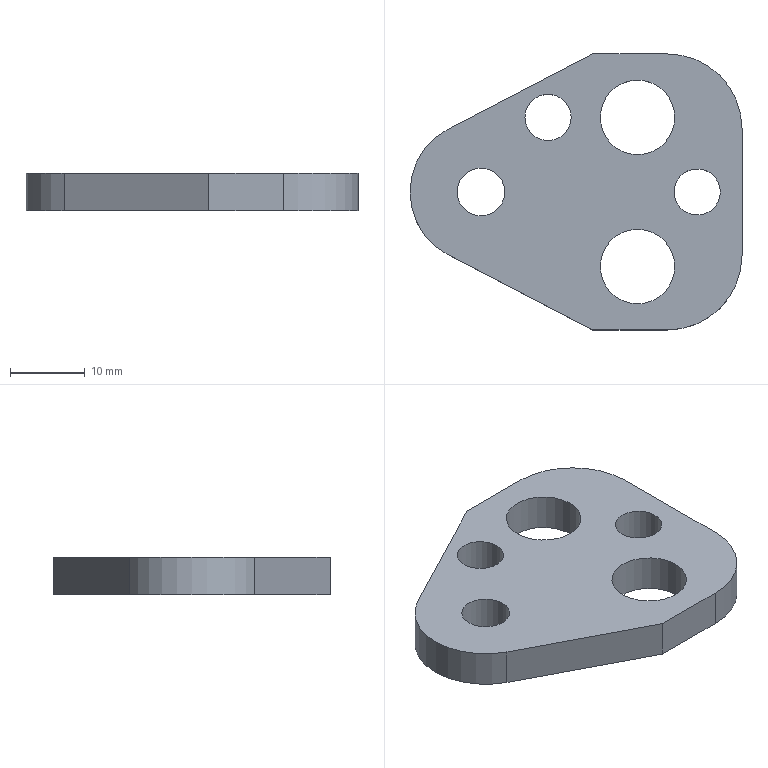Part | NX | features solid 2 | 1 solid | 15 faces | box 44.5 x 37 x 5 mm | volume 5155 mm3 | cylinder 8 | plane 7 | commonest cylinder face diameters 6.2 x2 10 x2 20 x2 6.4 x1 19 x1
STEP:
#1=CARTESIAN_POINT('',(-659.495,-526.443,93.));
#2=VERTEX_POINT('',#1);
#3=CARTESIAN_POINT('',(-649.495,-536.443,93.));
#4=VERTEX_POINT('',#3);
#5=CARTESIAN_POINT('',(-659.495,-536.443,93.));
#6=DIRECTION('',(0.,0.,-1.));
#7=DIRECTION('',(1.,0.,0.));
#8=AXIS2_PLACEMENT_3D('',#5,#6,#7);
#9=CIRCLE('',#8,10.);
#10=EDGE_CURVE('',#2,#4,#9,.T.);
#11=ORIENTED_EDGE('',*,*,#10,.F.);
#12=CARTESIAN_POINT('',(-659.495,-526.443,98.));
#13=VERTEX_POINT('',#12);
#14=CARTESIAN_POINT('',(-659.495,-526.443,98.));
#15=DIRECTION('',(0.,0.,-1.));
#16=VECTOR('',#15,1000.);
#17=LINE('',#14,#16);
#18=EDGE_CURVE('',#13,#2,#17,.T.);
#19=ORIENTED_EDGE('',*,*,#18,.F.);
#20=CARTESIAN_POINT('',(-649.495,-536.443,98.));
#21=VERTEX_POINT('',#20);
#22=CARTESIAN_POINT('',(-659.495,-536.443,98.));
#23=DIRECTION('',(0.,0.,-1.));
#24=DIRECTION('',(1.,0.,0.));
#25=AXIS2_PLACEMENT_3D('',#22,#23,#24);
#26=CIRCLE('',#25,10.);
#27=EDGE_CURVE('',#13,#21,#26,.T.);
#28=ORIENTED_EDGE('',*,*,#27,.T.);
#29=CARTESIAN_POINT('',(-649.495,-536.443,98.));
#30=DIRECTION('',(0.,0.,-1.));
#31=VECTOR('',#30,1000.);
#32=LINE('',#29,#31);
#33=EDGE_CURVE('',#21,#4,#32,.T.);
#34=ORIENTED_EDGE('',*,*,#33,.T.);
#35=EDGE_LOOP('',(#11,#19,#28,#34));
#36=FACE_BOUND('',#35,.T.);
#37=CARTESIAN_POINT('',(-659.495,-536.443,98.));
#38=DIRECTION('',(0.,0.,-1.));
#39=DIRECTION('',(1.,0.,0.));
#40=AXIS2_PLACEMENT_3D('',#37,#38,#39);
#41=CYLINDRICAL_SURFACE('',#40,10.);
#42=ADVANCED_FACE('',(#36),#41,.T.);
#43=CARTESIAN_POINT('',(-649.495,-553.443,93.));
#44=VERTEX_POINT('',#43);
#45=CARTESIAN_POINT('',(-649.495,-553.443,93.));
#46=DIRECTION('',(0.,1.,0.));
#47=VECTOR('',#46,1000.);
#48=LINE('',#45,#47);
#49=EDGE_CURVE('',#44,#4,#48,.T.);
#50=ORIENTED_EDGE('',*,*,#49,.T.);
#51=ORIENTED_EDGE('',*,*,#33,.F.);
#52=CARTESIAN_POINT('',(-649.495,-553.443,98.));
#53=VERTEX_POINT('',#52);
#54=CARTESIAN_POINT('',(-649.495,-553.443,98.));
#55=DIRECTION('',(0.,1.,0.));
#56=VECTOR('',#55,1000.);
#57=LINE('',#54,#56);
#58=EDGE_CURVE('',#53,#21,#57,.T.);
#59=ORIENTED_EDGE('',*,*,#58,.F.);
#60=CARTESIAN_POINT('',(-649.495,-553.443,98.));
#61=DIRECTION('',(0.,0.,-1.));
#62=VECTOR('',#61,1000.);
#63=LINE('',#60,#62);
#64=EDGE_CURVE('',#53,#44,#63,.T.);
#65=ORIENTED_EDGE('',*,*,#64,.T.);
#66=EDGE_LOOP('',(#50,#51,#59,#65));
#67=FACE_BOUND('',#66,.T.);
#68=CARTESIAN_POINT('',(-649.495,-553.443,98.));
#69=DIRECTION('',(-1.,0.,0.));
#70=DIRECTION('',(0.,-1.,0.));
#71=AXIS2_PLACEMENT_3D('',#68,#69,#70);
#72=PLANE('',#71);
#73=ADVANCED_FACE('',(#67),#72,.F.);
#74=CARTESIAN_POINT('',(-659.495,-563.443,93.));
#75=VERTEX_POINT('',#74);
#76=CARTESIAN_POINT('',(-659.495,-553.443,93.));
#77=DIRECTION('',(0.,0.,-1.));
#78=DIRECTION('',(1.,0.,0.));
#79=AXIS2_PLACEMENT_3D('',#76,#77,#78);
#80=CIRCLE('',#79,10.);
#81=EDGE_CURVE('',#44,#75,#80,.T.);
#82=ORIENTED_EDGE('',*,*,#81,.F.);
#83=ORIENTED_EDGE('',*,*,#64,.F.);
#84=CARTESIAN_POINT('',(-659.495,-563.443,98.));
#85=VERTEX_POINT('',#84);
#86=CARTESIAN_POINT('',(-659.495,-553.443,98.));
#87=DIRECTION('',(0.,0.,-1.));
#88=DIRECTION('',(1.,0.,0.));
#89=AXIS2_PLACEMENT_3D('',#86,#87,#88);
#90=CIRCLE('',#89,10.);
#91=EDGE_CURVE('',#53,#85,#90,.T.);
#92=ORIENTED_EDGE('',*,*,#91,.T.);
#93=CARTESIAN_POINT('',(-659.495,-563.443,98.));
#94=DIRECTION('',(0.,0.,-1.));
#95=VECTOR('',#94,1000.);
#96=LINE('',#93,#95);
#97=EDGE_CURVE('',#85,#75,#96,.T.);
#98=ORIENTED_EDGE('',*,*,#97,.T.);
#99=EDGE_LOOP('',(#82,#83,#92,#98));
#100=FACE_BOUND('',#99,.T.);
#101=CARTESIAN_POINT('',(-659.495,-553.443,98.));
#102=DIRECTION('',(0.,0.,-1.));
#103=DIRECTION('',(1.,0.,0.));
#104=AXIS2_PLACEMENT_3D('',#101,#102,#103);
#105=CYLINDRICAL_SURFACE('',#104,10.);
#106=ADVANCED_FACE('',(#100),#105,.T.);
#107=CARTESIAN_POINT('',(-669.495,-563.443,93.));
#108=VERTEX_POINT('',#107);
#109=CARTESIAN_POINT('',(-669.495,-563.443,93.));
#110=DIRECTION('',(1.,0.,0.));
#111=VECTOR('',#110,1000.);
#112=LINE('',#109,#111);
#113=EDGE_CURVE('',#108,#75,#112,.T.);
#114=ORIENTED_EDGE('',*,*,#113,.T.);
#115=ORIENTED_EDGE('',*,*,#97,.F.);
#116=CARTESIAN_POINT('',(-669.495,-563.443,98.));
#117=VERTEX_POINT('',#116);
#118=CARTESIAN_POINT('',(-669.495,-563.443,98.));
#119=DIRECTION('',(1.,0.,0.));
#120=VECTOR('',#119,1000.);
#121=LINE('',#118,#120);
#122=EDGE_CURVE('',#117,#85,#121,.T.);
#123=ORIENTED_EDGE('',*,*,#122,.F.);
#124=CARTESIAN_POINT('',(-669.495,-563.443,98.));
#125=DIRECTION('',(0.,0.,-1.));
#126=VECTOR('',#125,1000.);
#127=LINE('',#124,#126);
#128=EDGE_CURVE('',#117,#108,#127,.T.);
#129=ORIENTED_EDGE('',*,*,#128,.T.);
#130=EDGE_LOOP('',(#114,#115,#123,#129));
#131=FACE_BOUND('',#130,.T.);
#132=CARTESIAN_POINT('',(-669.495,-563.443,98.));
#133=DIRECTION('',(0.,1.,0.));
#134=DIRECTION('',(-1.,0.,0.));
#135=AXIS2_PLACEMENT_3D('',#132,#133,#134);
#136=PLANE('',#135);
#137=ADVANCED_FACE('',(#131),#136,.F.);
#138=CARTESIAN_POINT('',(-688.875,-553.373,93.));
#139=VERTEX_POINT('',#138);
#140=CARTESIAN_POINT('',(-688.875,-553.373,93.));
#141=DIRECTION('',(0.8874,-0.4611,0.));
#142=VECTOR('',#141,1000.);
#143=LINE('',#140,#142);
#144=EDGE_CURVE('',#139,#108,#143,.T.);
#145=ORIENTED_EDGE('',*,*,#144,.T.);
#146=ORIENTED_EDGE('',*,*,#128,.F.);
#147=CARTESIAN_POINT('',(-688.875,-553.373,98.));
#148=VERTEX_POINT('',#147);
#149=CARTESIAN_POINT('',(-688.875,-553.373,98.));
#150=DIRECTION('',(0.8874,-0.4611,0.));
#151=VECTOR('',#150,1000.);
#152=LINE('',#149,#151);
#153=EDGE_CURVE('',#148,#117,#152,.T.);
#154=ORIENTED_EDGE('',*,*,#153,.F.);
#155=CARTESIAN_POINT('',(-688.875,-553.373,98.));
#156=DIRECTION('',(0.,0.,-1.));
#157=VECTOR('',#156,1000.);
#158=LINE('',#155,#157);
#159=EDGE_CURVE('',#148,#139,#158,.T.);
#160=ORIENTED_EDGE('',*,*,#159,.T.);
#161=EDGE_LOOP('',(#145,#146,#154,#160));
#162=FACE_BOUND('',#161,.T.);
#163=CARTESIAN_POINT('',(-688.875,-553.373,98.));
#164=DIRECTION('',(0.4611,0.8874,0.));
#165=DIRECTION('',(-0.8874,0.4611,0.));
#166=AXIS2_PLACEMENT_3D('',#163,#164,#165);
#167=PLANE('',#166);
#168=ADVANCED_FACE('',(#162),#167,.F.);
#169=CARTESIAN_POINT('',(-688.875,-536.513,93.));
#170=VERTEX_POINT('',#169);
#171=CARTESIAN_POINT('',(-684.495,-544.943,93.));
#172=DIRECTION('',(0.,0.,-1.));
#173=DIRECTION('',(1.,0.,0.));
#174=AXIS2_PLACEMENT_3D('',#171,#172,#173);
#175=CIRCLE('',#174,9.5);
#176=EDGE_CURVE('',#139,#170,#175,.T.);
#177=ORIENTED_EDGE('',*,*,#176,.F.);
#178=ORIENTED_EDGE('',*,*,#159,.F.);
#179=CARTESIAN_POINT('',(-688.875,-536.513,98.));
#180=VERTEX_POINT('',#179);
#181=CARTESIAN_POINT('',(-684.495,-544.943,98.));
#182=DIRECTION('',(0.,0.,-1.));
#183=DIRECTION('',(1.,0.,0.));
#184=AXIS2_PLACEMENT_3D('',#181,#182,#183);
#185=CIRCLE('',#184,9.5);
#186=EDGE_CURVE('',#148,#180,#185,.T.);
#187=ORIENTED_EDGE('',*,*,#186,.T.);
#188=CARTESIAN_POINT('',(-688.875,-536.513,98.));
#189=DIRECTION('',(0.,0.,-1.));
#190=VECTOR('',#189,1000.);
#191=LINE('',#188,#190);
#192=EDGE_CURVE('',#180,#170,#191,.T.);
#193=ORIENTED_EDGE('',*,*,#192,.T.);
#194=EDGE_LOOP('',(#177,#178,#187,#193));
#195=FACE_BOUND('',#194,.T.);
#196=CARTESIAN_POINT('',(-684.495,-544.943,98.));
#197=DIRECTION('',(0.,0.,-1.));
#198=DIRECTION('',(1.,0.,0.));
#199=AXIS2_PLACEMENT_3D('',#196,#197,#198);
#200=CYLINDRICAL_SURFACE('',#199,9.5);
#201=ADVANCED_FACE('',(#195),#200,.T.);
#202=CARTESIAN_POINT('',(-669.495,-526.443,93.));
#203=VERTEX_POINT('',#202);
#204=CARTESIAN_POINT('',(-688.875,-536.513,93.));
#205=DIRECTION('',(0.8874,0.4611,0.));
#206=VECTOR('',#205,1000.);
#207=LINE('',#204,#206);
#208=EDGE_CURVE('',#170,#203,#207,.T.);
#209=ORIENTED_EDGE('',*,*,#208,.F.);
#210=ORIENTED_EDGE('',*,*,#192,.F.);
#211=CARTESIAN_POINT('',(-669.495,-526.443,98.));
#212=VERTEX_POINT('',#211);
#213=CARTESIAN_POINT('',(-688.875,-536.513,98.));
#214=DIRECTION('',(0.8874,0.4611,0.));
#215=VECTOR('',#214,1000.);
#216=LINE('',#213,#215);
#217=EDGE_CURVE('',#180,#212,#216,.T.);
#218=ORIENTED_EDGE('',*,*,#217,.T.);
#219=CARTESIAN_POINT('',(-669.495,-526.443,98.));
#220=DIRECTION('',(0.,0.,-1.));
#221=VECTOR('',#220,1000.);
#222=LINE('',#219,#221);
#223=EDGE_CURVE('',#212,#203,#222,.T.);
#224=ORIENTED_EDGE('',*,*,#223,.T.);
#225=EDGE_LOOP('',(#209,#210,#218,#224));
#226=FACE_BOUND('',#225,.T.);
#227=CARTESIAN_POINT('',(-688.875,-536.513,98.));
#228=DIRECTION('',(-0.4611,0.8874,0.));
#229=DIRECTION('',(-0.8874,-0.4611,0.));
#230=AXIS2_PLACEMENT_3D('',#227,#228,#229);
#231=PLANE('',#230);
#232=ADVANCED_FACE('',(#226),#231,.T.);
#233=CARTESIAN_POINT('',(-669.495,-526.443,93.));
#234=DIRECTION('',(1.,0.,0.));
#235=VECTOR('',#234,1000.);
#236=LINE('',#233,#235);
#237=EDGE_CURVE('',#203,#2,#236,.T.);
#238=ORIENTED_EDGE('',*,*,#237,.F.);
#239=ORIENTED_EDGE('',*,*,#223,.F.);
#240=CARTESIAN_POINT('',(-669.495,-526.443,98.));
#241=DIRECTION('',(1.,0.,0.));
#242=VECTOR('',#241,1000.);
#243=LINE('',#240,#242);
#244=EDGE_CURVE('',#212,#13,#243,.T.);
#245=ORIENTED_EDGE('',*,*,#244,.T.);
#246=ORIENTED_EDGE('',*,*,#18,.T.);
#247=EDGE_LOOP('',(#238,#239,#245,#246));
#248=FACE_BOUND('',#247,.T.);
#249=CARTESIAN_POINT('',(-669.495,-526.443,98.));
#250=DIRECTION('',(0.,1.,0.));
#251=DIRECTION('',(-1.,0.,0.));
#252=AXIS2_PLACEMENT_3D('',#249,#250,#251);
#253=PLANE('',#252);
#254=ADVANCED_FACE('',(#248),#253,.T.);
#255=CARTESIAN_POINT('',(-658.495,-554.943,98.));
#256=VERTEX_POINT('',#255);
#257=CARTESIAN_POINT('',(-663.495,-554.943,98.));
#258=DIRECTION('',(0.,0.,-1.));
#259=DIRECTION('',(1.,0.,0.));
#260=AXIS2_PLACEMENT_3D('',#257,#258,#259);
#261=CIRCLE('',#260,5.);
#262=EDGE_CURVE('',#256,#256,#261,.T.);
#263=ORIENTED_EDGE('',*,*,#262,.T.);
#264=EDGE_LOOP('',(#263));
#265=FACE_BOUND('',#264,.T.);
#266=CARTESIAN_POINT('',(-658.495,-534.943,98.));
#267=VERTEX_POINT('',#266);
#268=CARTESIAN_POINT('',(-663.495,-534.943,98.));
#269=DIRECTION('',(0.,0.,-1.));
#270=DIRECTION('',(1.,0.,0.));
#271=AXIS2_PLACEMENT_3D('',#268,#269,#270);
#272=CIRCLE('',#271,5.);
#273=EDGE_CURVE('',#267,#267,#272,.T.);
#274=ORIENTED_EDGE('',*,*,#273,.T.);
#275=EDGE_LOOP('',(#274));
#276=FACE_BOUND('',#275,.T.);
#277=CARTESIAN_POINT('',(-681.295,-544.943,98.));
#278=VERTEX_POINT('',#277);
#279=CARTESIAN_POINT('',(-684.495,-544.943,98.));
#280=DIRECTION('',(0.,0.,-1.));
#281=DIRECTION('',(1.,0.,0.));
#282=AXIS2_PLACEMENT_3D('',#279,#280,#281);
#283=CIRCLE('',#282,3.2);
#284=EDGE_CURVE('',#278,#278,#283,.T.);
#285=ORIENTED_EDGE('',*,*,#284,.T.);
#286=EDGE_LOOP('',(#285));
#287=FACE_BOUND('',#286,.T.);
#288=CARTESIAN_POINT('',(-672.395,-534.943,98.));
#289=VERTEX_POINT('',#288);
#290=CARTESIAN_POINT('',(-675.495,-534.943,98.));
#291=DIRECTION('',(0.,0.,-1.));
#292=DIRECTION('',(1.,0.,0.));
#293=AXIS2_PLACEMENT_3D('',#290,#291,#292);
#294=CIRCLE('',#293,3.1);
#295=EDGE_CURVE('',#289,#289,#294,.T.);
#296=ORIENTED_EDGE('',*,*,#295,.T.);
#297=EDGE_LOOP('',(#296));
#298=FACE_BOUND('',#297,.T.);
#299=CARTESIAN_POINT('',(-652.395,-544.943,98.));
#300=VERTEX_POINT('',#299);
#301=CARTESIAN_POINT('',(-655.495,-544.943,98.));
#302=DIRECTION('',(0.,0.,-1.));
#303=DIRECTION('',(1.,0.,0.));
#304=AXIS2_PLACEMENT_3D('',#301,#302,#303);
#305=CIRCLE('',#304,3.1);
#306=EDGE_CURVE('',#300,#300,#305,.T.);
#307=ORIENTED_EDGE('',*,*,#306,.T.);
#308=EDGE_LOOP('',(#307));
#309=FACE_BOUND('',#308,.T.);
#310=ORIENTED_EDGE('',*,*,#27,.F.);
#311=ORIENTED_EDGE('',*,*,#244,.F.);
#312=ORIENTED_EDGE('',*,*,#217,.F.);
#313=ORIENTED_EDGE('',*,*,#186,.F.);
#314=ORIENTED_EDGE('',*,*,#153,.T.);
#315=ORIENTED_EDGE('',*,*,#122,.T.);
#316=ORIENTED_EDGE('',*,*,#91,.F.);
#317=ORIENTED_EDGE('',*,*,#58,.T.);
#318=EDGE_LOOP('',(#310,#311,#312,#313,#314,#315,#316,#317));
#319=FACE_BOUND('',#318,.T.);
#320=CARTESIAN_POINT('',(-659.495,-536.443,98.));
#321=DIRECTION('',(0.,0.,-1.));
#322=DIRECTION('',(1.,0.,0.));
#323=AXIS2_PLACEMENT_3D('',#320,#321,#322);
#324=PLANE('',#323);
#325=ADVANCED_FACE('',(#265,#276,#287,#298,#309,#319),#324,.F.);
#326=CARTESIAN_POINT('',(-658.495,-554.943,93.));
#327=VERTEX_POINT('',#326);
#328=CARTESIAN_POINT('',(-663.495,-554.943,93.));
#329=DIRECTION('',(0.,0.,-1.));
#330=DIRECTION('',(1.,0.,0.));
#331=AXIS2_PLACEMENT_3D('',#328,#329,#330);
#332=CIRCLE('',#331,5.);
#333=EDGE_CURVE('',#327,#327,#332,.T.);
#334=ORIENTED_EDGE('',*,*,#333,.F.);
#335=EDGE_LOOP('',(#334));
#336=FACE_BOUND('',#335,.T.);
#337=CARTESIAN_POINT('',(-658.495,-534.943,93.));
#338=VERTEX_POINT('',#337);
#339=CARTESIAN_POINT('',(-663.495,-534.943,93.));
#340=DIRECTION('',(0.,0.,-1.));
#341=DIRECTION('',(1.,0.,0.));
#342=AXIS2_PLACEMENT_3D('',#339,#340,#341);
#343=CIRCLE('',#342,5.);
#344=EDGE_CURVE('',#338,#338,#343,.T.);
#345=ORIENTED_EDGE('',*,*,#344,.F.);
#346=EDGE_LOOP('',(#345));
#347=FACE_BOUND('',#346,.T.);
#348=CARTESIAN_POINT('',(-681.295,-544.943,93.));
#349=VERTEX_POINT('',#348);
#350=CARTESIAN_POINT('',(-684.495,-544.943,93.));
#351=DIRECTION('',(0.,0.,-1.));
#352=DIRECTION('',(1.,0.,0.));
#353=AXIS2_PLACEMENT_3D('',#350,#351,#352);
#354=CIRCLE('',#353,3.2);
#355=EDGE_CURVE('',#349,#349,#354,.T.);
#356=ORIENTED_EDGE('',*,*,#355,.F.);
#357=EDGE_LOOP('',(#356));
#358=FACE_BOUND('',#357,.T.);
#359=CARTESIAN_POINT('',(-672.395,-534.943,93.));
#360=VERTEX_POINT('',#359);
#361=CARTESIAN_POINT('',(-675.495,-534.943,93.));
#362=DIRECTION('',(0.,0.,-1.));
#363=DIRECTION('',(1.,0.,0.));
#364=AXIS2_PLACEMENT_3D('',#361,#362,#363);
#365=CIRCLE('',#364,3.1);
#366=EDGE_CURVE('',#360,#360,#365,.T.);
#367=ORIENTED_EDGE('',*,*,#366,.F.);
#368=EDGE_LOOP('',(#367));
#369=FACE_BOUND('',#368,.T.);
#370=CARTESIAN_POINT('',(-652.395,-544.943,93.));
#371=VERTEX_POINT('',#370);
#372=CARTESIAN_POINT('',(-655.495,-544.943,93.));
#373=DIRECTION('',(0.,0.,-1.));
#374=DIRECTION('',(1.,0.,0.));
#375=AXIS2_PLACEMENT_3D('',#372,#373,#374);
#376=CIRCLE('',#375,3.1);
#377=EDGE_CURVE('',#371,#371,#376,.T.);
#378=ORIENTED_EDGE('',*,*,#377,.F.);
#379=EDGE_LOOP('',(#378));
#380=FACE_BOUND('',#379,.T.);
#381=ORIENTED_EDGE('',*,*,#10,.T.);
#382=ORIENTED_EDGE('',*,*,#49,.F.);
#383=ORIENTED_EDGE('',*,*,#81,.T.);
#384=ORIENTED_EDGE('',*,*,#113,.F.);
#385=ORIENTED_EDGE('',*,*,#144,.F.);
#386=ORIENTED_EDGE('',*,*,#176,.T.);
#387=ORIENTED_EDGE('',*,*,#208,.T.);
#388=ORIENTED_EDGE('',*,*,#237,.T.);
#389=EDGE_LOOP('',(#381,#382,#383,#384,#385,#386,#387,#388));
#390=FACE_BOUND('',#389,.T.);
#391=CARTESIAN_POINT('',(-659.495,-536.443,93.));
#392=DIRECTION('',(0.,0.,-1.));
#393=DIRECTION('',(1.,0.,0.));
#394=AXIS2_PLACEMENT_3D('',#391,#392,#393);
#395=PLANE('',#394);
#396=ADVANCED_FACE('',(#336,#347,#358,#369,#380,#390),#395,.T.);
#397=ORIENTED_EDGE('',*,*,#377,.T.);
#398=EDGE_LOOP('',(#397));
#399=FACE_BOUND('',#398,.T.);
#400=ORIENTED_EDGE('',*,*,#306,.F.);
#401=EDGE_LOOP('',(#400));
#402=FACE_BOUND('',#401,.T.);
#403=CARTESIAN_POINT('',(-655.495,-544.943,98.));
#404=DIRECTION('',(0.,0.,-1.));
#405=DIRECTION('',(1.,0.,0.));
#406=AXIS2_PLACEMENT_3D('',#403,#404,#405);
#407=CYLINDRICAL_SURFACE('',#406,3.1);
#408=ADVANCED_FACE('',(#399,#402),#407,.F.);
#409=ORIENTED_EDGE('',*,*,#366,.T.);
#410=EDGE_LOOP('',(#409));
#411=FACE_BOUND('',#410,.T.);
#412=ORIENTED_EDGE('',*,*,#295,.F.);
#413=EDGE_LOOP('',(#412));
#414=FACE_BOUND('',#413,.T.);
#415=CARTESIAN_POINT('',(-675.495,-534.943,98.));
#416=DIRECTION('',(0.,0.,-1.));
#417=DIRECTION('',(1.,0.,0.));
#418=AXIS2_PLACEMENT_3D('',#415,#416,#417);
#419=CYLINDRICAL_SURFACE('',#418,3.1);
#420=ADVANCED_FACE('',(#411,#414),#419,.F.);
#421=ORIENTED_EDGE('',*,*,#355,.T.);
#422=EDGE_LOOP('',(#421));
#423=FACE_BOUND('',#422,.T.);
#424=ORIENTED_EDGE('',*,*,#284,.F.);
#425=EDGE_LOOP('',(#424));
#426=FACE_BOUND('',#425,.T.);
#427=CARTESIAN_POINT('',(-684.495,-544.943,98.));
#428=DIRECTION('',(0.,0.,-1.));
#429=DIRECTION('',(1.,0.,0.));
#430=AXIS2_PLACEMENT_3D('',#427,#428,#429);
#431=CYLINDRICAL_SURFACE('',#430,3.2);
#432=ADVANCED_FACE('',(#423,#426),#431,.F.);
#433=ORIENTED_EDGE('',*,*,#344,.T.);
#434=EDGE_LOOP('',(#433));
#435=FACE_BOUND('',#434,.T.);
#436=ORIENTED_EDGE('',*,*,#273,.F.);
#437=EDGE_LOOP('',(#436));
#438=FACE_BOUND('',#437,.T.);
#439=CARTESIAN_POINT('',(-663.495,-534.943,98.));
#440=DIRECTION('',(0.,0.,-1.));
#441=DIRECTION('',(1.,0.,0.));
#442=AXIS2_PLACEMENT_3D('',#439,#440,#441);
#443=CYLINDRICAL_SURFACE('',#442,5.);
#444=ADVANCED_FACE('',(#435,#438),#443,.F.);
#445=ORIENTED_EDGE('',*,*,#333,.T.);
#446=EDGE_LOOP('',(#445));
#447=FACE_BOUND('',#446,.T.);
#448=ORIENTED_EDGE('',*,*,#262,.F.);
#449=EDGE_LOOP('',(#448));
#450=FACE_BOUND('',#449,.T.);
#451=CARTESIAN_POINT('',(-663.495,-554.943,98.));
#452=DIRECTION('',(0.,0.,-1.));
#453=DIRECTION('',(1.,0.,0.));
#454=AXIS2_PLACEMENT_3D('',#451,#452,#453);
#455=CYLINDRICAL_SURFACE('',#454,5.);
#456=ADVANCED_FACE('',(#447,#450),#455,.F.);
#457=CLOSED_SHELL('',(#42,#73,#106,#137,#168,#201,#232,#254,#325,#396,#408,#420,#432,#444,#456));
#458=MANIFOLD_SOLID_BREP('',#457);
#459=(LENGTH_UNIT()NAMED_UNIT(*)SI_UNIT(.MILLI.,.METRE.));
#460=UNCERTAINTY_MEASURE_WITH_UNIT(LENGTH_MEASURE(0.00001),#459,'','');
#461=(NAMED_UNIT(*)PLANE_ANGLE_UNIT()SI_UNIT($,.RADIAN.));
#462=(NAMED_UNIT(*)SI_UNIT($,.STERADIAN.)SOLID_ANGLE_UNIT());
#463=(GEOMETRIC_REPRESENTATION_CONTEXT(3)GLOBAL_UNCERTAINTY_ASSIGNED_CONTEXT((#460))GLOBAL_UNIT_ASSIGNED_CONTEXT((#459,#461,#462))REPRESENTATION_CONTEXT('',''));
#464=ADVANCED_BREP_SHAPE_REPRESENTATION('',(#458),#463);